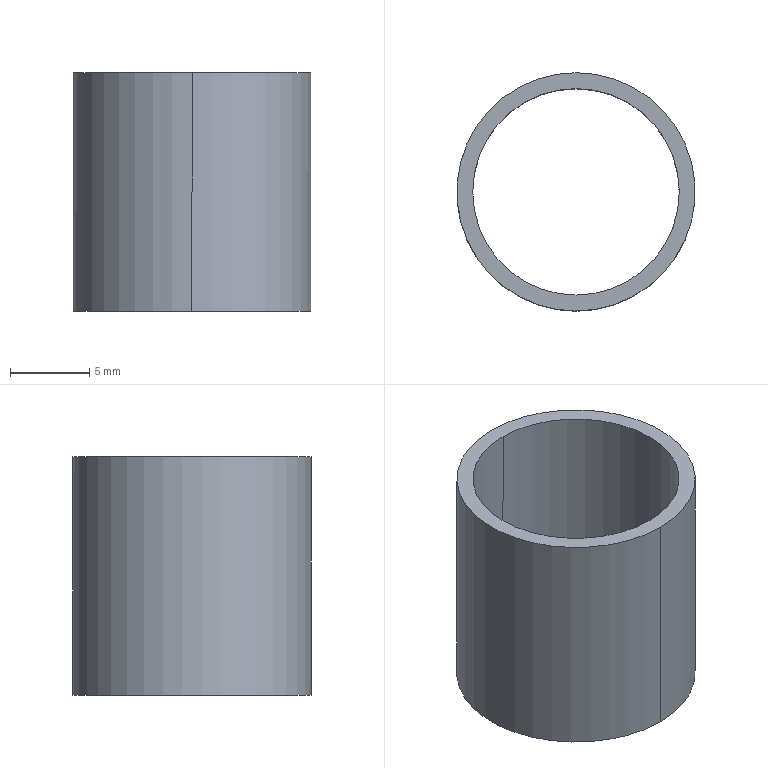Part | SolidWorks | features BaseBody 1 | 1 solid | 6 faces | box 15.004 x 15.002 x 15.005 mm | volume 659.734 mm3 | cylinder 4 | plane 2 | commonest cylinder face diameters 13 x2 15 x2
STEP:
#1=CARTESIAN_POINT('',(406.069,-9.211,53.586));
#2=VERTEX_POINT('',#1);
#3=CARTESIAN_POINT('',(406.069,-22.211,53.584));
#4=VERTEX_POINT('',#3);
#5=CARTESIAN_POINT('',(406.069,-15.711,53.585));
#6=DIRECTION('',(0.0002857,-0.0001428,1.));
#7=DIRECTION('',(0.000000041,1.,0.0001428));
#8=AXIS2_PLACEMENT_3D('',#5,#6,#7);
#9=CIRCLE('',#8,6.5);
#10=EDGE_CURVE('',#2,#4,#9,.T.);
#11=ORIENTED_EDGE('',*,*,#10,.F.);
#12=CARTESIAN_POINT('',(406.073,-9.213,68.586));
#13=VERTEX_POINT('',#12);
#14=CARTESIAN_POINT('',(406.069,-9.211,53.586));
#15=DIRECTION('',(0.0002857,-0.0001428,1.));
#16=VECTOR('',#15,1000.);
#17=LINE('',#14,#16);
#18=EDGE_CURVE('',#2,#13,#17,.T.);
#19=ORIENTED_EDGE('',*,*,#18,.T.);
#20=CARTESIAN_POINT('',(406.073,-22.213,68.584));
#21=VERTEX_POINT('',#20);
#22=CARTESIAN_POINT('',(406.073,-15.713,68.585));
#23=DIRECTION('',(-0.0002857,0.0001428,-1.));
#24=DIRECTION('',(1.,0.,-0.0002857));
#25=AXIS2_PLACEMENT_3D('',#22,#23,#24);
#26=CIRCLE('',#25,6.5);
#27=EDGE_CURVE('',#21,#13,#26,.T.);
#28=ORIENTED_EDGE('',*,*,#27,.F.);
#29=CARTESIAN_POINT('',(406.069,-22.211,53.584));
#30=DIRECTION('',(0.0002857,-0.0001428,1.));
#31=VECTOR('',#30,1000.);
#32=LINE('',#29,#31);
#33=EDGE_CURVE('',#4,#21,#32,.T.);
#34=ORIENTED_EDGE('',*,*,#33,.F.);
#35=EDGE_LOOP('',(#11,#19,#28,#34));
#36=FACE_OUTER_BOUND('',#35,.T.);
#37=CARTESIAN_POINT('',(406.069,-15.711,53.585));
#38=DIRECTION('',(0.0002857,-0.0001428,1.));
#39=DIRECTION('',(-0.000000041,-1.,-0.0001428));
#40=AXIS2_PLACEMENT_3D('',#37,#38,#39);
#41=CYLINDRICAL_SURFACE('',#40,6.5);
#42=ADVANCED_FACE('',(#36),#41,.F.);
#43=CARTESIAN_POINT('',(406.069,-8.211,53.586));
#44=VERTEX_POINT('',#43);
#45=CARTESIAN_POINT('',(406.069,-23.211,53.584));
#46=VERTEX_POINT('',#45);
#47=CARTESIAN_POINT('',(406.069,-15.711,53.585));
#48=DIRECTION('',(-0.0002857,0.0001428,-1.));
#49=DIRECTION('',(-0.000000041,-1.,-0.0001428));
#50=AXIS2_PLACEMENT_3D('',#47,#48,#49);
#51=CIRCLE('',#50,7.5);
#52=EDGE_CURVE('',#44,#46,#51,.T.);
#53=ORIENTED_EDGE('',*,*,#52,.F.);
#54=CARTESIAN_POINT('',(406.073,-8.213,68.586));
#55=VERTEX_POINT('',#54);
#56=CARTESIAN_POINT('',(406.069,-8.211,53.586));
#57=DIRECTION('',(0.0002857,-0.0001428,1.));
#58=VECTOR('',#57,1000.);
#59=LINE('',#56,#58);
#60=EDGE_CURVE('',#44,#55,#59,.T.);
#61=ORIENTED_EDGE('',*,*,#60,.T.);
#62=CARTESIAN_POINT('',(406.073,-23.213,68.584));
#63=VERTEX_POINT('',#62);
#64=CARTESIAN_POINT('',(406.073,-15.713,68.585));
#65=DIRECTION('',(0.0002857,-0.0001428,1.));
#66=DIRECTION('',(-0.000000041,-1.,-0.0001428));
#67=AXIS2_PLACEMENT_3D('',#64,#65,#66);
#68=CIRCLE('',#67,7.5);
#69=EDGE_CURVE('',#63,#55,#68,.T.);
#70=ORIENTED_EDGE('',*,*,#69,.F.);
#71=CARTESIAN_POINT('',(406.069,-23.211,53.584));
#72=DIRECTION('',(0.0002857,-0.0001428,1.));
#73=VECTOR('',#72,1000.);
#74=LINE('',#71,#73);
#75=EDGE_CURVE('',#46,#63,#74,.T.);
#76=ORIENTED_EDGE('',*,*,#75,.F.);
#77=EDGE_LOOP('',(#53,#61,#70,#76));
#78=FACE_OUTER_BOUND('',#77,.T.);
#79=CARTESIAN_POINT('',(406.069,-15.711,53.585));
#80=DIRECTION('',(0.0002857,-0.0001428,1.));
#81=DIRECTION('',(-0.000000041,-1.,-0.0001428));
#82=AXIS2_PLACEMENT_3D('',#79,#80,#81);
#83=CYLINDRICAL_SURFACE('',#82,7.5);
#84=ADVANCED_FACE('',(#78),#83,.T.);
#85=ORIENTED_EDGE('',*,*,#60,.F.);
#86=CARTESIAN_POINT('',(406.069,-15.711,53.585));
#87=DIRECTION('',(-0.0002857,0.0001428,-1.));
#88=DIRECTION('',(-0.000000041,-1.,-0.0001428));
#89=AXIS2_PLACEMENT_3D('',#86,#87,#88);
#90=CIRCLE('',#89,7.5);
#91=EDGE_CURVE('',#46,#44,#90,.T.);
#92=ORIENTED_EDGE('',*,*,#91,.F.);
#93=ORIENTED_EDGE('',*,*,#75,.T.);
#94=CARTESIAN_POINT('',(406.073,-15.713,68.585));
#95=DIRECTION('',(0.0002857,-0.0001428,1.));
#96=DIRECTION('',(-0.000000041,-1.,-0.0001428));
#97=AXIS2_PLACEMENT_3D('',#94,#95,#96);
#98=CIRCLE('',#97,7.5);
#99=EDGE_CURVE('',#55,#63,#98,.T.);
#100=ORIENTED_EDGE('',*,*,#99,.F.);
#101=EDGE_LOOP('',(#85,#92,#93,#100));
#102=FACE_OUTER_BOUND('',#101,.T.);
#103=CARTESIAN_POINT('',(406.069,-15.711,53.585));
#104=DIRECTION('',(0.0002857,-0.0001428,1.));
#105=DIRECTION('',(-0.000000041,-1.,-0.0001428));
#106=AXIS2_PLACEMENT_3D('',#103,#104,#105);
#107=CYLINDRICAL_SURFACE('',#106,7.5);
#108=ADVANCED_FACE('',(#102),#107,.T.);
#109=ORIENTED_EDGE('',*,*,#27,.T.);
#110=CARTESIAN_POINT('',(406.073,-15.713,68.585));
#111=DIRECTION('',(-0.0002857,0.0001428,-1.));
#112=DIRECTION('',(1.,0.,-0.0002857));
#113=AXIS2_PLACEMENT_3D('',#110,#111,#112);
#114=CIRCLE('',#113,6.5);
#115=EDGE_CURVE('',#13,#21,#114,.T.);
#116=ORIENTED_EDGE('',*,*,#115,.T.);
#117=EDGE_LOOP('',(#109,#116));
#118=FACE_BOUND('',#117,.T.);
#119=ORIENTED_EDGE('',*,*,#69,.T.);
#120=ORIENTED_EDGE('',*,*,#99,.T.);
#121=EDGE_LOOP('',(#119,#120));
#122=FACE_OUTER_BOUND('',#121,.T.);
#123=CARTESIAN_POINT('',(406.073,-15.713,68.585));
#124=DIRECTION('',(0.0002857,-0.0001428,1.));
#125=DIRECTION('',(-0.4472,-0.8944,0.));
#126=AXIS2_PLACEMENT_3D('',#123,#124,#125);
#127=PLANE('',#126);
#128=ADVANCED_FACE('',(#118,#122),#127,.T.);
#129=ORIENTED_EDGE('',*,*,#18,.F.);
#130=CARTESIAN_POINT('',(406.069,-15.711,53.585));
#131=DIRECTION('',(0.0002857,-0.0001428,1.));
#132=DIRECTION('',(0.000000041,1.,0.0001428));
#133=AXIS2_PLACEMENT_3D('',#130,#131,#132);
#134=CIRCLE('',#133,6.5);
#135=EDGE_CURVE('',#4,#2,#134,.T.);
#136=ORIENTED_EDGE('',*,*,#135,.F.);
#137=ORIENTED_EDGE('',*,*,#33,.T.);
#138=ORIENTED_EDGE('',*,*,#115,.F.);
#139=EDGE_LOOP('',(#129,#136,#137,#138));
#140=FACE_OUTER_BOUND('',#139,.T.);
#141=CARTESIAN_POINT('',(406.069,-15.711,53.585));
#142=DIRECTION('',(0.0002857,-0.0001428,1.));
#143=DIRECTION('',(-0.000000041,-1.,-0.0001428));
#144=AXIS2_PLACEMENT_3D('',#141,#142,#143);
#145=CYLINDRICAL_SURFACE('',#144,6.5);
#146=ADVANCED_FACE('',(#140),#145,.F.);
#147=ORIENTED_EDGE('',*,*,#135,.T.);
#148=ORIENTED_EDGE('',*,*,#10,.T.);
#149=EDGE_LOOP('',(#147,#148));
#150=FACE_BOUND('',#149,.T.);
#151=ORIENTED_EDGE('',*,*,#91,.T.);
#152=ORIENTED_EDGE('',*,*,#52,.T.);
#153=EDGE_LOOP('',(#151,#152));
#154=FACE_OUTER_BOUND('',#153,.T.);
#155=CARTESIAN_POINT('',(406.069,-15.711,53.585));
#156=DIRECTION('',(0.0002857,-0.0001428,1.));
#157=DIRECTION('',(-0.4472,-0.8944,0.));
#158=AXIS2_PLACEMENT_3D('',#155,#156,#157);
#159=PLANE('',#158);
#160=ADVANCED_FACE('',(#150,#154),#159,.F.);
#161=CLOSED_SHELL('',(#42,#84,#108,#128,#146,#160));
#162=MANIFOLD_SOLID_BREP('',#161);
#163=CARTESIAN_POINT('',(0.,0.,0.));
#164=DIRECTION('',(0.,0.,1.));
#165=DIRECTION('',(1.,0.,0.));
#166=AXIS2_PLACEMENT_3D('',#163,#164,#165);
#167=(LENGTH_UNIT()NAMED_UNIT(*)SI_UNIT(.MILLI.,.METRE.));
#168=UNCERTAINTY_MEASURE_WITH_UNIT(LENGTH_MEASURE(0.00001),#167,'','');
#169=(NAMED_UNIT(*)PLANE_ANGLE_UNIT()SI_UNIT($,.RADIAN.));
#170=(NAMED_UNIT(*)SI_UNIT($,.STERADIAN.)SOLID_ANGLE_UNIT());
#171=(GEOMETRIC_REPRESENTATION_CONTEXT(3)GLOBAL_UNCERTAINTY_ASSIGNED_CONTEXT((#168))GLOBAL_UNIT_ASSIGNED_CONTEXT((#167,#169,#170))REPRESENTATION_CONTEXT('',''));
#172=ADVANCED_BREP_SHAPE_REPRESENTATION('',(#162,#166),#171);